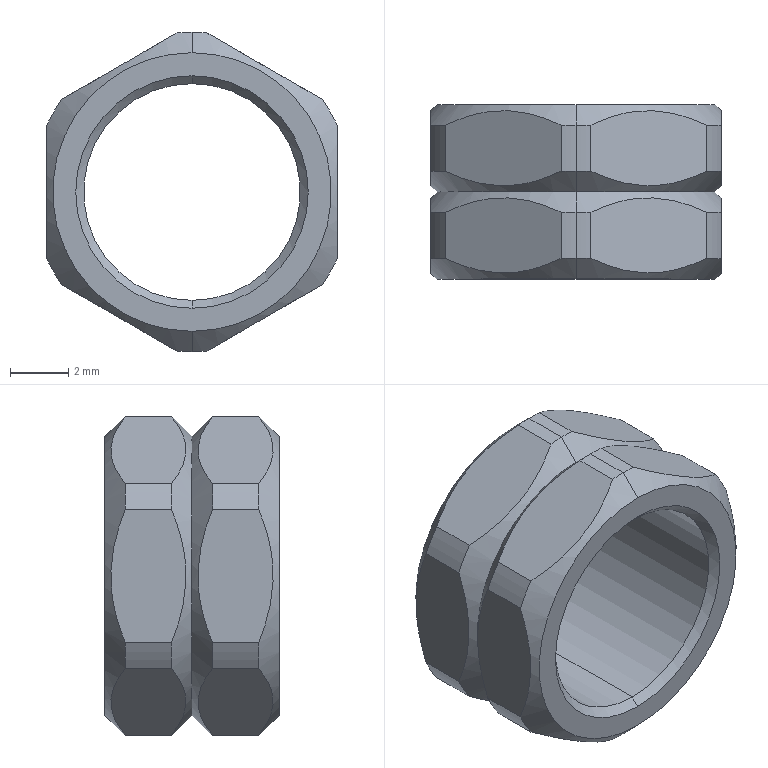Part | SolidWorks | features BaseBody 1 | 1 solid | 42 faces | box 10 x 6 x 11 mm | volume 236.508 mm3 | cylinder 16 | plane 14 | cone 12 | commonest cylinder face diameters 11 x14 7.459 x2